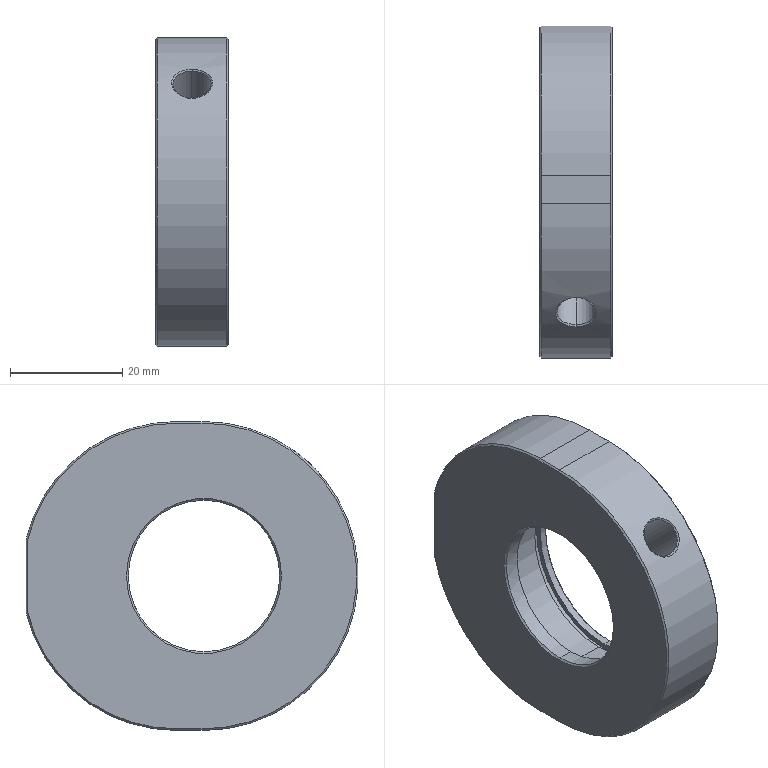Part | STEP file | opening-closing seat_SUS304 | 1 solid | 39 faces | box 13 x 59.2 x 55 mm | volume 24027 mm3 | plane 14 | cylinder 13 | cone 10 | spline 2 | commonest cylinder face diameters 32 x4 55 x3 6.8 x2 27 x2 33.9 x2